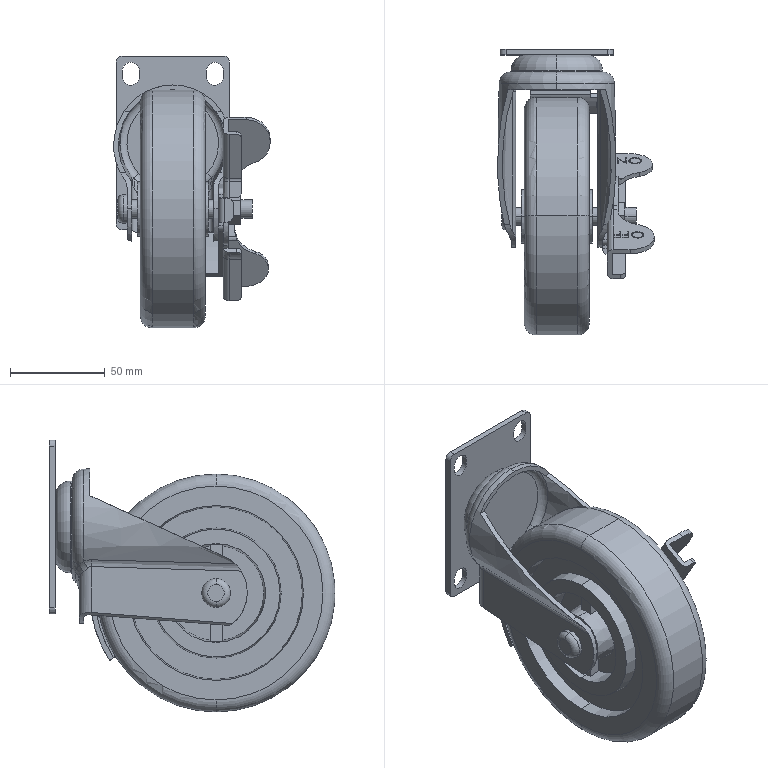Part | SolidWorks | features AEMSimFeature 1, CompositeCurve 1 | 6 solids | 328 faces | box 82.741 x 151.003 x 143.701 mm | volume 434028 mm3 | plane 151 | cylinder 84 | spline 43 | torus 28 | cone 22 | commonest cylinder face diameters 6.35 x20 9.017 x12 5.08 x6 25.4 x6 9.525 x4 11.112 x4